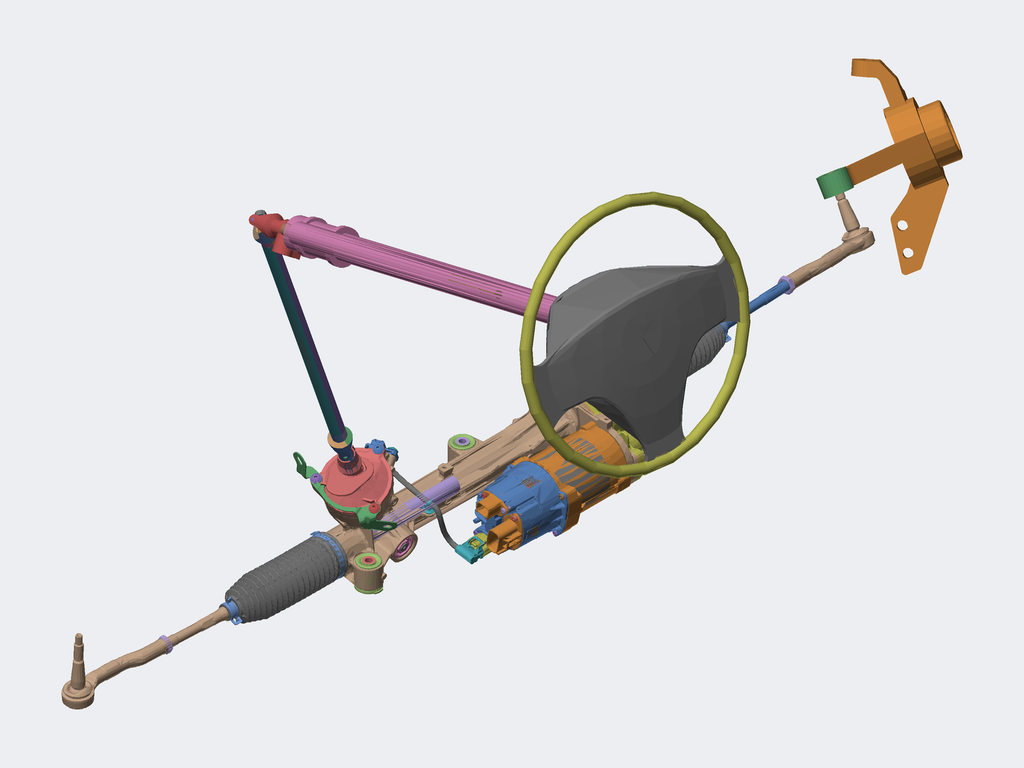Assembly | SolidWorks | 247 different items | 250 placed
Parts list (item | name | quantity | size | volume | features):
1 | - | x1 | 19.402 x 3.35 x 11.935 mm | 493.088 mm3 | features BaseBody 1
2 | - | x1 | 30 x 26.016 x 30 mm | 2608 mm3 | features BaseBody 1
3 | - | x1 | 4.5 x 4.5 x 4.5 mm | 47.713 mm3 | features BaseBody 1
4 | - | x1 | 34.044 x 0.2 x 37.494 mm | 39.583 mm3 | features BaseBody 1
5 | - | x1 | 5.111 x 7.707 x 11.846 mm | 71.275 mm3 | features BaseBody 1
6 | - | x1 | 4.732 x 5.384 x 5.638 mm | 55.081 mm3 | features BaseBody 1
7 | - | x1 | 4.732 x 5.384 x 5.638 mm | 55.081 mm3 | features BaseBody 1
8 | - | x1 | 84.752 x 78.463 x 43.87 mm | 1584 mm3 | features BaseBody 1
9 | - | x1 | 74.696 x 74 x 74.696 mm | 200799 mm3 | features BaseBody 1
10 | - | x1 | 0.3505 x 1.273 x 1.232 mm | 0.05013 mm3 | features BaseBody 1
11 | - | x1 | 0.9771 x 0.8707 x 1.35 mm | 0.03036 mm3 | features BaseBody 1
12 | - | x1 | 1.687 x 95.5 x 0.9097 mm | 85.989 mm3 | features BaseBody 1
13 | - | x1 | 44.117 x 78.054 x 132.466 mm | 28853 mm3 | features BaseBody 1
14 | - | x1 | 0.7417 x 0.8074 x 1.179 mm | 0.04503 mm3 | features BaseBody 1
15 | - | x1 | 1.687 x 95.5 x 0.9097 mm | 85.97 mm3 | features BaseBody 1
16 | - | x1 | 5.111 x 7.707 x 11.846 mm | 71.275 mm3 | features BaseBody 1
17 | - | x1 | 29.983 x 29.981 x 20.298 mm | 2883 mm3 | features BaseBody 1
18 | - | x1 | 35 x 35 x 41.7 mm | 8862 mm3 | features BaseBody 1
19 | - | x1 | 9.725 x 10.19 x 8.66 mm | 146.52 mm3 | features BaseBody 1
20 | - | x1 | 40 x 47.036 x 40 mm | 19515 mm3 | features BaseBody 1
21 | - | x1 | 36.383 x 52.2 x 58.261 mm | 12719 mm3 | features BaseBody 1
22 | - | x1 | 127.966 x 60.952 x 91.962 mm | 4231 mm3 | features BaseBody 1
23 | - | x1 | 20.099 x 66.9 x 5.857 mm | 673.523 mm3 | features BaseBody 1
24 | - | x1 | 16.002 x 15.682 x 17 mm | 610.766 mm3 | features BaseBody 1
25 | - | x1 | 8 x 14.81 x 8 mm | 243.858 mm3 | features BaseBody 1
26 | - | x1 | 21.746 x 3 x 7.946 mm | 278.91 mm3 | features BaseBody 1
27 | - | x1 | 1.687 x 95.5 x 0.9097 mm | 85.989 mm3 | features BaseBody 1
28 | - | x1 | 4.5 x 4.5 x 4.5 mm | 47.713 mm3 | features BaseBody 1
29 | - | x1 | 15.957 x 12 x 12.696 mm | 692.518 mm3 | features BaseBody 1
30 | - | x1 | 7 x 12.8 x 7 mm | 210.469 mm3 | features BaseBody 1
31 | - | x1 | 46 x 5.6 x 46 mm | 1252 mm3 | features BaseBody 1
32 | - | x1 | 16.862 x 11.769 x 16.004 mm | 237.71 mm3 | features BaseBody 1
33 | - | x1 | 34.658 x 35.361 x 27.908 mm | 375.706 mm3 | features BaseBody 1
34 | - | x1 | 14.55 x 34.479 x 14.55 mm | 1284 mm3 | features BaseBody 1
35 | - | x1 | 22.149 x 20.875 x 12.86 mm | 64.48 mm3 | features BaseBody 1
36 | - | x1 | 4.5 x 4.5 x 4.5 mm | 47.713 mm3 | features BaseBody 1
37 | - | x1 | 5.111 x 7.707 x 11.846 mm | 71.275 mm3 | features BaseBody 1
38 | - | x1 | 57.96 x 1.78 x 57.96 mm | 439.199 mm3 | features BaseBody 1
39 | - | x1 | 5.111 x 7.707 x 11.846 mm | 71.275 mm3 | features BaseBody 1
40 | - | x1 | 29.254 x 28.081 x 18.745 mm | 719.848 mm3 | features BaseBody 1
41 | - | x1 | 15.622 x 10.059 x 16.879 mm | 251.42 mm3 | features BaseBody 1
42 | - | x1 | 9.466 x 6.792 x 10.714 mm | 122.784 mm3 | features BaseBody 1
43 | - | x1 | 4.5 x 4.5 x 4.5 mm | 47.713 mm3 | features BaseBody 1
44 | - | x1 | 14.289 x 18.177 x 23.78 mm | 994.304 mm3 | features BaseBody 1
45 | - | x1 | 10.992 x 29 x 22.904 mm | 695.627 mm3 | features BaseBody 1
46 | - | x1 | 29.5 x 15.5 x 29.5 mm | 2238 mm3 | features BaseBody 1
47 | - | x1 | 22.954 x 22.595 x 15.926 mm | 80.609 mm3 | features BaseBody 1
48 | - | x1 | 4.732 x 5.384 x 5.638 mm | 55.081 mm3 | features BaseBody 1
49 | - | x1 | 4.768 x 5.451 x 5.709 mm | 55.187 mm3 | features BaseBody 1
50 | - | x1 | 16.092 x 16.511 x 27.057 mm | 643.939 mm3 | features BaseBody 1
51 | - | x1 | 0.4319 x 1.035 x 1.185 mm | 0.04699 mm3 | features BaseBody 1
52 | - | x1 | 4.732 x 5.384 x 5.638 mm | 55.081 mm3 | features BaseBody 1
53 | - | x1 | 0.5835 x 1.422 x 1.475 mm | 0.05932 mm3 | features BaseBody 1
54 | - | x1 | 0.3903 x 1.163 x 1.223 mm | 0.04564 mm3 | features BaseBody 1
55 | - | x1 | 14.752 x 4.1 x 6.976 mm | 179.488 mm3 | features BaseBody 1
56 | - | x1 | 67.591 x 179.747 x 65.54 mm | 46175 mm3 | features BaseBody 1
57 | - | x1 | 40.908 x 40.949 x 3.578 mm | 397.302 mm3 | features BaseBody 1
58 | - | x1 | 40 x 36 x 39.5 mm | 12667 mm3 | features BaseBody 1
59 | - | x1 | 9.725 x 10.19 x 8.66 mm | 146.52 mm3 | features BaseBody 1
60 | - | x1 | 42.008 x 239.227 x 32.291 mm | 49739 mm3 | features BaseBody 1
61 | - | x1 | 42.008 x 239.227 x 32.309 mm | 49735 mm3 | features MBimport 1
62 | - | x1 | 4.732 x 5.384 x 5.638 mm | 55.081 mm3 | features BaseBody 1
63 | - | x1 | 20.926 x 45.783 x 18.973 mm | 386.348 mm3 | features BaseBody 1
64 | - | x1 | 36.9 x 4.5 x 36.885 mm | 1647 mm3 | features BaseBody 1
65 | - | x1 | 0.9706 x 0.8253 x 1.218 mm | 0.04974 mm3 | features BaseBody 1
66 | - | x1 | 0.379 x 1.595 x 1.505 mm | 0.06995 mm3 | features BaseBody 1
67 | - | x1 | 47.8 x 15.1 x 47.8 mm | 5914 mm3 | features BaseBody 1
68 | - | x1 | 1.595 x 0.8611 x 1.514 mm | 0.04844 mm3 | features BaseBody 1
69 | - | x1 | 1.687 x 95.5 x 0.9097 mm | 85.97 mm3 | features BaseBody 1
70 | - | x1 | 41.506 x 41.869 x 24.152 mm | 5595 mm3 | features BaseBody 1
71 | - | x1 | 25.1 x 25.07 x 2.979 mm | 184.393 mm3 | features BaseBody 1
72 | - | x1 | 102.773 x 118.28 x 97.783 mm | 55614 mm3 | features BaseBody 1
73 | - | x1 | 4.5 x 4.5 x 4.5 mm | 47.713 mm3 | features BaseBody 1
74 | - | x1 | 24.623 x 9.204 x 21.336 mm | 1841 mm3 | features BaseBody 1
75 | - | x1 | 41.492 x 163.305 x 30.52 mm | 40087 mm3 | features BaseBody 1
76 | - | x1 | 8 x 14.81 x 8 mm | 243.858 mm3 | features BaseBody 1
77 | - | x1 | 1.687 x 95.5 x 0.9097 mm | 85.97 mm3 | features BaseBody 1
78 | - | x1 | 16.532 x 22.966 x 18.857 mm | 994.304 mm3 | features BaseBody 1
79 | - | x1 | 16.984 x 9.25 x 11.199 mm | 695.298 mm3 | features BaseBody 1
80 | - | x1 | 26.743 x 0.2 x 14.919 mm | 22.901 mm3 | features BaseBody 1
81 | - | x1 | 30 x 26.016 x 30 mm | 2608 mm3 | features BaseBody 1
82 | - | x1 | 8 x 14.81 x 8 mm | 243.858 mm3 | features BaseBody 1
83 | - | x1 | 1.687 x 95.5 x 0.9097 mm | 85.989 mm3 | features BaseBody 1
84 | - | x1 | 9.855 x 34.04 x 33.526 mm | 478.172 mm3 | features BaseBody 1
85 | - | x1 | 7 x 12.8 x 7 mm | 210.469 mm3 | features BaseBody 1
86 | - | x1 | 43 x 5.5 x 43 mm | 1963 mm3 | features BaseBody 1
87 | - | x1 | 31.818 x 23.75 x 20.928 mm | 3737 mm3 | features BaseBody 1
88 | - | x1 | 14.55 x 24.44 x 14.55 mm | 994.304 mm3 | features BaseBody 1
89 | - | x1 | 73.281 x 73.868 x 57.617 mm | 92633 mm3 | features BaseBody 1
90 | - | x1 | 5.111 x 7.707 x 11.846 mm | 71.275 mm3 | features BaseBody 1
91 | - | x1 | 36.983 x 37.484 x 29.782 mm | 1472 mm3 | features BaseBody 1
92 | - | x1 | 4.5 x 4.5 x 4.5 mm | 47.713 mm3 | features BaseBody 1
93 | - | x1 | 1.687 x 95.5 x 0.9097 mm | 85.97 mm3 | features BaseBody 1
94 | - | x1 | 8 x 14.81 x 8 mm | 243.858 mm3 | features BaseBody 1
95 | - | x1 | 5.111 x 7.707 x 11.846 mm | 71.275 mm3 | features BaseBody 1
96 | - | x1 | 16.219 x 17.338 x 12.294 mm | 776.179 mm3 | features BaseBody 1
97 | - | x1 | 32.369 x 32.817 x 25.668 mm | 6352 mm3 | features BaseBody 1
98 | - | x1 | 5.111 x 7.707 x 11.846 mm | 71.275 mm3 | features BaseBody 1
99 | - | x1 | 5.111 x 7.707 x 11.846 mm | 71.275 mm3 | features BaseBody 1
100 | - | x1 | 63 x 7 x 63.493 mm | 1084 mm3 | features BaseBody 1
101 | - | x1 | 14.289 x 18.177 x 23.78 mm | 994.304 mm3 | features BaseBody 1
102 | - | x1 | 27.136 x 25.603 x 15.645 mm | 211.754 mm3 | features BaseBody 1
103 | - | x1 | 4.732 x 5.384 x 5.638 mm | 55.081 mm3 | features BaseBody 1
104 | - | x1 | 4.732 x 5.384 x 5.638 mm | 55.081 mm3 | features BaseBody 1
105 | - | x1 | 1.687 x 95.5 x 0.9097 mm | 85.989 mm3 | features BaseBody 1
106 | - | x1 | 17.995 x 23.635 x 17.388 mm | 1594 mm3 | features BaseBody 1
107 | - | x1 | 36.9 x 4.5 x 36.885 mm | 1648 mm3 | features BaseBody 1
108 | - | x1 | 0.6733 x 1.06 x 1.265 mm | 0.03834 mm3 | features BaseBody 1
109 | - | x1 | 0.4717 x 1.454 x 1.483 mm | 0.06327 mm3 | features BaseBody 1
110 | - | x1 | 0.9414 x 1.02 x 1.363 mm | 0.04689 mm3 | features BaseBody 1
111 | - | x1 | 29.543 x 30.33 x 21.946 mm | 3664 mm3 | features BaseBody 1
112 | - | x1 | 5.111 x 7.707 x 11.846 mm | 71.275 mm3 | features BaseBody 1
113 | - | x1 | 41.509 x 41.866 x 24.145 mm | 5595 mm3 | features BaseBody 1
114 | - | x1 | 40.908 x 40.949 x 3.578 mm | 397.302 mm3 | features BaseBody 1
115 | - | x1 | 40 x 36 x 39.5 mm | 12667 mm3 | features BaseBody 1
116 | - | x1 | 0.3887 x 0.7999 x 1.186 mm | 0.02402 mm3 | features BaseBody 1
117 | - | x1 | 40 x 47.036 x 40 mm | 19515 mm3 | features BaseBody 1
118 | - | x1 | 19.061 x 36 x 36.564 mm | 8491 mm3 | features BaseBody 1
119 | - | x2 | 25 x 25 x 101.883 mm | 19881 mm3 | features BaseBody 1
120 | - | x1 | 1.687 x 95.5 x 0.9097 mm | 85.989 mm3 | features BaseBody 1
121 | - | x1 | 11.583 x 19.87 x 24.283 mm | 2380 mm3 | features BaseBody 1
122 | - | x1 | 1.687 x 95.5 x 0.9097 mm | 85.989 mm3 | features BaseBody 1
123 | - | x1 | 31.731 x 29.251 x 16.171 mm | 110.749 mm3 | features BaseBody 1
124 | - | x1 | 1.687 x 95.5 x 0.9097 mm | 85.989 mm3 | features BaseBody 1
125 | - | x1 | 8 x 14.81 x 8 mm | 243.858 mm3 | features BaseBody 1
126 | - | x1 | 2.721 x 20 x 14.787 mm | 30.051 mm3 | features BaseBody 1
127 | - | x1 | 9.855 x 34.04 x 33.526 mm | 478.172 mm3 | features BaseBody 1
128 | - | x1 | 67.591 x 179.747 x 65.54 mm | 46179 mm3 | features BaseBody 1
129 | - | x1 | 60.43 x 1.78 x 60.43 mm | 458.509 mm3 | features BaseBody 1
130 | - | x1 | 7 x 12.8 x 7 mm | 210.469 mm3 | features BaseBody 1
131 | - | x1 | 14.5 x 44.401 x 14.5 mm | 1558 mm3 | features BaseBody 1
132 | - | x1 | 28.804 x 28.259 x 20.047 mm | 1513 mm3 | features BaseBody 1
133 | - | x1 | 31.483 x 14.462 x 33.309 mm | 1146 mm3 | features BaseBody 1
134 | - | x1 | 127.707 x 25 x 70 mm | 11936 mm3 | features BaseBody 1
135 | - | x1 | 5.111 x 7.707 x 11.846 mm | 71.275 mm3 | features BaseBody 1
136 | - | x1 | 35.944 x 33.77 x 20.198 mm | 291.989 mm3 | features BaseBody 1
137 | - | x1 | 4.5 x 4.5 x 4.5 mm | 47.713 mm3 | features BaseBody 1
138 | - | x1 | 13.105 x 13.906 x 12.577 mm | 373.199 mm3 | features BaseBody 1
139 | - | x1 | 28.907 x 12 x 30 mm | 1841 mm3 | features BaseBody 1
140 | - | x1 | 5.111 x 7.707 x 11.846 mm | 71.275 mm3 | features BaseBody 1
141 | - | x1 | 5.111 x 7.707 x 11.846 mm | 71.275 mm3 | features BaseBody 1
142 | - | x1 | 47.8 x 15.1 x 47.8 mm | 5914 mm3 | features BaseBody 1
143 | - | x1 | 9.592 x 5.588 x 11.054 mm | 19.29 mm3 | features BaseBody 1
144 | - | x1 | 29.233 x 27.963 x 17.759 mm | 697.835 mm3 | features BaseBody 1
145 | - | x1 | 5.111 x 7.707 x 11.846 mm | 71.275 mm3 | features BaseBody 1
146 | - | x1 | 4.732 x 5.384 x 5.638 mm | 55.081 mm3 | features BaseBody 1
147 | - | x1 | 4.732 x 5.384 x 5.638 mm | 55.081 mm3 | features BaseBody 1
148 | - | x1 | 109.447 x 62.133 x 148.234 mm | 8333 mm3 | features BaseBody 1
149 | - | x1 | - | 242474 mm3 | features BaseBody 1
150 | - | x1 | 0.631 x 1.244 x 1.435 mm | 0.04371 mm3 | features BaseBody 1
151 | - | x1 | 0.6157 x 1.809 x 1.538 mm | 0.08303 mm3 | features BaseBody 1
152 | - | x1 | 1.15 x 0.8105 x 1.338 mm | 0.03304 mm3 | features BaseBody 1
153 | - | x1 | 43.345 x 65.256 x 106.487 mm | 42238 mm3 | features BaseBody 1
154 | - | x1 | 266.066 x 277.183 x 171.657 mm | 646593 mm3 | features MBimport 1
155 | - | x1 | 47 x 41 x 79 mm | 34473 mm3 | features MBimport 1
156 | - | x1 | 5.111 x 7.707 x 11.846 mm | 71.275 mm3 | features BaseBody 1
157 | - | x1 | - | - | features MBimport 1
158 | - | x1 | 34 x 6.427 x 34 mm | 1749 mm3 | features MBimport 1
159 | - | x1 | 366 x 115.12 x 366 mm | 3175003 mm3 | features MBimport 1
160 | - | x1 | 430 x 46 x 46 mm | 92426 mm3 | features MBimport 1
161 | - | x1 | 580 x 52.513 x 52.513 mm | 240293 mm3 | features MBimport 1
162 | - | x1 | 44 x 38 x 42 mm | 20383 mm3 | features MBimport 1
163 | - | x1 | 14.289 x 18.177 x 23.78 mm | 994.304 mm3 | features BaseBody 1
164 | - | x1 | 5.111 x 7.707 x 11.846 mm | 71.275 mm3 | features BaseBody 1
165 | - | x1 | 14.5 x 44.401 x 14.5 mm | 1558 mm3 | features BaseBody 1
166 | - | x1 | 9.876 x 13.68 x 6.803 mm | 39.142 mm3 | features BaseBody 1
167 | - | x1 | 5.111 x 7.707 x 11.846 mm | 71.275 mm3 | features BaseBody 1
168 | - | x1 | 25.1 x 25.07 x 2.981 mm | 184.393 mm3 | features BaseBody 1
169 | - | x1 | 4.732 x 5.384 x 5.638 mm | 55.081 mm3 | features BaseBody 1
170 | - | x1 | 4.732 x 5.384 x 5.638 mm | 55.081 mm3 | features BaseBody 1
171 | - | x1 | 85 x 162.58 x 85 mm | 554074 mm3 | features BaseBody 1
172 | - | x1 | 32.722 x 59.616 x 108.746 mm | 4991 mm3 | features BaseBody 1
173 | - | x1 | 0.6045 x 1.069 x 1.25 mm | 0.05056 mm3 | features BaseBody 1
174 | - | x1 | 22.149 x 20.875 x 12.86 mm | 64.468 mm3 | features BaseBody 1
175 | - | x1 | 8.65 x 8.202 x 5.272 mm | 36.271 mm3 | features BaseBody 1
176 | - | x1 | 13.154 x 13.951 x 12.601 mm | 373.279 mm3 | features BaseBody 1
177 | - | x1 | 31.952 x 32.01 x 7.031 mm | 1769 mm3 | features BaseBody 1
178 | - | x1 | 40 x 36 x 39.5 mm | 12667 mm3 | features BaseBody 1
179 | - | x1 | 35 x 35 x 41.7 mm | 8862 mm3 | features BaseBody 1
180 | - | x1 | 31.952 x 32.01 x 7.026 mm | 1769 mm3 | features BaseBody 1
181 | - | x2 | 24.623 x 9.204 x 21.336 mm | 1841 mm3 | features BaseBody 1
182 | - | x2 | 41.492 x 163.306 x 30.502 mm | 40065 mm3 | features BaseBody 1
183 | - | x1 | 49.369 x 96.8 x 21.617 mm | 9085 mm3 | features BaseBody 1
184 | - | x1 | 1.687 x 95.5 x 0.9097 mm | 85.989 mm3 | features BaseBody 1
185 | - | x1 | 16.985 x 9.25 x 11.204 mm | 695.298 mm3 | features BaseBody 1
186 | - | x1 | 18.588 x 19.086 x 15.342 mm | 855.538 mm3 | features BaseBody 1
187 | - | x1 | 10.728 x 19.45 x 9.871 mm | 648.732 mm3 | features BaseBody 1
188 | - | x1 | 8 x 14.81 x 8 mm | 243.858 mm3 | features BaseBody 1
189 | - | x1 | 8 x 14.81 x 8 mm | 243.858 mm3 | features BaseBody 1
190 | - | x1 | 3.855 x 5.685 x 6.743 mm | 2.538 mm3 | features BaseBody 1
191 | - | x1 | 35.548 x 33.98 x 39.287 mm | 16613 mm3 | features BaseBody 1
192 | - | x1 | 5.31 x 6 x 6.631 mm | 70.058 mm3 | features BaseBody 1
193 | - | x1 | 46 x 5.6 x 46 mm | 1252 mm3 | features BaseBody 1
194 | - | x1 | 14.55 x 34.479 x 14.55 mm | 1284 mm3 | features BaseBody 1
195 | - | x1 | 5.111 x 7.707 x 11.846 mm | 71.275 mm3 | features BaseBody 1
196 | - | x1 | 31.483 x 14.462 x 33.309 mm | 1146 mm3 | features BaseBody 1
197 | - | x1 | 5.111 x 7.707 x 11.846 mm | 71.275 mm3 | features BaseBody 1
198 | - | x1 | 8 x 14.81 x 8 mm | 243.858 mm3 | features BaseBody 1
199 | - | x1 | 36.935 x 34.817 x 21.16 mm | 1456 mm3 | features BaseBody 1
200 | - | x1 | 5.111 x 7.707 x 11.846 mm | 71.275 mm3 | features BaseBody 1
201 | - | x1 | 42.008 x 239.227 x 32.291 mm | 49739 mm3 | features BaseBody 1
202 | - | x1 | 5.111 x 7.707 x 11.846 mm | 71.275 mm3 | features BaseBody 1
203 | - | x1 | 57.96 x 1.78 x 57.96 mm | 439.199 mm3 | features BaseBody 1
204 | - | x1 | 4.5 x 4.5 x 4.5 mm | 47.713 mm3 | features BaseBody 1
205 | - | x1 | 4.5 x 4.5 x 4.5 mm | 47.713 mm3 | features BaseBody 1
206 | - | x1 | 4.5 x 4.5 x 4.5 mm | 47.713 mm3 | features BaseBody 1
207 | - | x1 | 16.505 x 16.005 x 17.799 mm | 676.72 mm3 | features BaseBody 1
208 | - | x1 | 4.732 x 5.384 x 5.638 mm | 55.081 mm3 | features BaseBody 1
209 | - | x1 | 4.732 x 5.384 x 5.638 mm | 55.081 mm3 | features BaseBody 1
210 | - | x1 | 32.672 x 30.577 x 18.335 mm | 710.143 mm3 | features BaseBody 1
211 | - | x1 | 85 x 56.019 x 85 mm | 176710 mm3 | features BaseBody 1
212 | - | x1 | 1.687 x 95.5 x 0.9097 mm | 85.97 mm3 | features BaseBody 1
213 | - | x1 | 0.6635 x 0.9504 x 1.207 mm | 0.04104 mm3 | features BaseBody 1
214 | - | x1 | 0.8136 x 0.9655 x 1.252 mm | 0.03857 mm3 | features BaseBody 1
215 | - | x1 | 0.8628 x 0.8341 x 1.199 mm | 0.04242 mm3 | features BaseBody 1
216 | - | x1 | 1.048 x 0.7769 x 1.387 mm | 0.03423 mm3 | features BaseBody 1
217 | - | x1 | 29.983 x 29.981 x 20.302 mm | 2883 mm3 | features BaseBody 1
218 | - | x1 | 35 x 35 x 41.7 mm | 8862 mm3 | features BaseBody 1
219 | - | x1 | 9.725 x 10.19 x 8.66 mm | 146.564 mm3 | features BaseBody 1
220 | - | x1 | 25.15 x 648.8 x 25.15 mm | 264219 mm3 | features BaseBody 1
221 | - | x1 | - | 689588 mm3 | features BaseBody 1
222 | - | x1 | 5.111 x 7.707 x 11.846 mm | 71.275 mm3 | features BaseBody 1
223 | - | x1 | 110.214 x 131 x 97.13 mm | 198684 mm3 | features BaseBody 1
224 | - | x1 | 25 x 25 x 101.883 mm | 19881 mm3 | features BaseBody 1
225 | - | x1 | 110.202 x 80.7 x 95 mm | 124997 mm3 | features BaseBody 1
226 | - | x1 | 45.461 x 98.495 x 26.021 mm | 9928 mm3 | features BaseBody 1
227 | - | x1 | 1.687 x 95.5 x 0.9097 mm | 85.989 mm3 | features BaseBody 1
228 | - | x1 | 1.687 x 95.5 x 0.9097 mm | 85.989 mm3 | features BaseBody 1
229 | - | x1 | 8 x 14.81 x 8 mm | 243.858 mm3 | features BaseBody 1
230 | - | x1 | 12.902 x 66.9 x 14.209 mm | 657.962 mm3 | features BaseBody 1
231 | - | x1 | 10.587 x 37.5 x 36.875 mm | 507.842 mm3 | features BaseBody 1
232 | - | x1 | 7 x 12.8 x 7 mm | 210.469 mm3 | features BaseBody 1
233 | - | x1 | 43 x 5.5 x 43 mm | 1963 mm3 | features BaseBody 1
234 | - | x1 | 15.479 x 20.6 x 6.702 mm | 129.141 mm3 | features BaseBody 1
235 | - | x1 | 151.361 x 3.9 x 96.963 mm | 2710 mm3 | features BaseBody 1
236 | - | x1 | 16.862 x 11.769 x 16.004 mm | 237.71 mm3 | features BaseBody 1
237 | - | x1 | 14.55 x 34.479 x 14.55 mm | 1284 mm3 | features BaseBody 1
238 | - | x1 | 63 x 7 x 63.493 mm | 1084 mm3 | features BaseBody 1
239 | - | x1 | 5.111 x 7.707 x 11.846 mm | 71.275 mm3 | features BaseBody 1
240 | - | x1 | 14.55 x 34.479 x 14.55 mm | 1284 mm3 | features BaseBody 1
241 | - | x1 | 5.111 x 7.707 x 11.846 mm | 71.275 mm3 | features BaseBody 1
242 | - | x1 | 5.111 x 7.707 x 11.846 mm | 71.275 mm3 | features BaseBody 1
243 | - | x1 | 44.308 x 41.304 x 38.03 mm | 10705 mm3 | features BaseBody 1
244 | - | x1 | 22.755 x 0.2 x 15.726 mm | 20.749 mm3 | features BaseBody 1
245 | - | x1 | 1.687 x 95.5 x 0.9097 mm | 85.97 mm3 | features BaseBody 1
246 | Symmetry of Symmetry of zhuan xiang jie hui zhi | x1 | - | - | -
247 | zhuan xiang jie hui zhi.step | x1 | - | - | -
Mates (type | each side: item.copy, entity, surface, feature):
Concentric | 60.1 face cylinder Input 1 | 181.1 face cylinder Input 1
Coincident | 182.1 face plane Input 1 | 181.1 face plane Input 1
Tangent | 182.1 face torus Input 1 | 119.1 face sphere Input 1
Coincident | 13.1 face plane Input 1 | 157.1 face plane wan xiang jie zhong zhou.CATPart<1> | 2 times
Concentric | 13.1 face cylinder Input 1 | 157.1 face cylinder wan xiang jie zhong zhou.CATPart<1>
Concentric | 157.1 face cylinder wan xiang jie zhong zhou.CATPart<1> | 158.1 face cylinder wan xiang jie shi zi zhou 2.CATPart<1>
Tangent | 157.1 face cylinder wan xiang jie zhong zhou.CATPart<1> | 158.1 face plane wan xiang jie shi zi zhou 2.CATPart<1>
Concentric | 155.1 face cylinder wan xiang jie shang jie tou.CATPart<1> | 158.1 face cylinder wan xiang jie shi zi zhou 2.CATPart<1>
Tangent | 155.1 face cylinder wan xiang jie shang jie tou.CATPart<1> | 158.1 face plane wan xiang jie shi zi zhou 2.CATPart<1>
Concentric | 155.1 face cylinder wan xiang jie shang jie tou.CATPart<1> | 160.1 face cylinder zhuan xiang zhu.CATPart<1>
Coincident | 155.1 face plane wan xiang jie shang jie tou.CATPart<1> | 160.1 face plane zhuan xiang zhu.CATPart<1>
Concentric | 160.1 face cylinder zhuan xiang zhu.CATPart<1> | 161.1 face cylinder zhuan xiang zhu tao tong.CATPart<1>
Coincident | 155.1 face plane wan xiang jie shang jie tou.CATPart<1> | 161.1 face plane zhuan xiang zhu tao tong.CATPart<1>
Coincident | 161.1 edge | 159.1 face cone fang xiang pan hui zhi.CATPart<1>